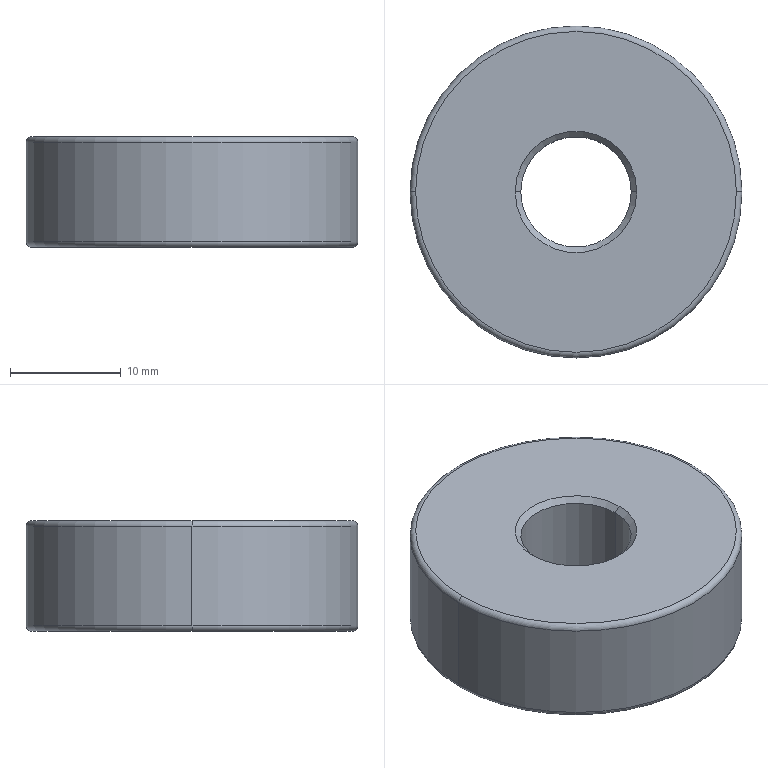Part | SolidWorks | features MirrorStock 1 | 1 solid | 14 faces | box 30 x 30 x 10 mm | volume 6265 mm3 | cone 4 | torus 4 | cylinder 4 | plane 2 | commonest cylinder face diameters 10 x2 30 x2
STEP:
#1=CARTESIAN_POINT('',(5.,0.,-9.5));
#2=VERTEX_POINT('',#1);
#3=CARTESIAN_POINT('',(-5.,0.,-9.5));
#4=VERTEX_POINT('',#3);
#5=CARTESIAN_POINT('',(0.,0.,-9.5));
#6=DIRECTION('',(0.,0.,1.));
#7=DIRECTION('',(1.,0.,0.));
#8=AXIS2_PLACEMENT_3D('',#5,#6,#7);
#9=CIRCLE('',#8,5.);
#10=EDGE_CURVE('',#2,#4,#9,.T.);
#11=ORIENTED_EDGE('',*,*,#10,.T.);
#12=CARTESIAN_POINT('',(-5.5,0.,-10.));
#13=VERTEX_POINT('',#12);
#14=CARTESIAN_POINT('',(-5.,0.,-9.5));
#15=DIRECTION('',(-0.7071,0.,-0.7071));
#16=VECTOR('',#15,1000.);
#17=LINE('',#14,#16);
#18=EDGE_CURVE('',#4,#13,#17,.T.);
#19=ORIENTED_EDGE('',*,*,#18,.T.);
#20=CARTESIAN_POINT('',(5.5,0.,-10.));
#21=VERTEX_POINT('',#20);
#22=CARTESIAN_POINT('',(0.,0.,-10.));
#23=DIRECTION('',(0.,0.,-1.));
#24=DIRECTION('',(1.,0.,0.));
#25=AXIS2_PLACEMENT_3D('',#22,#23,#24);
#26=CIRCLE('',#25,5.5);
#27=EDGE_CURVE('',#13,#21,#26,.T.);
#28=ORIENTED_EDGE('',*,*,#27,.T.);
#29=CARTESIAN_POINT('',(5.,0.,-9.5));
#30=DIRECTION('',(0.7071,0.,-0.7071));
#31=VECTOR('',#30,1000.);
#32=LINE('',#29,#31);
#33=EDGE_CURVE('',#2,#21,#32,.T.);
#34=ORIENTED_EDGE('',*,*,#33,.F.);
#35=EDGE_LOOP('',(#11,#19,#28,#34));
#36=FACE_OUTER_BOUND('',#35,.T.);
#37=CARTESIAN_POINT('',(0.,0.,-9.5));
#38=DIRECTION('',(0.,0.,-1.));
#39=DIRECTION('',(1.,0.,0.));
#40=AXIS2_PLACEMENT_3D('',#37,#38,#39);
#41=CONICAL_SURFACE('',#40,5.,0.7854);
#42=ADVANCED_FACE('',(#36),#41,.F.);
#43=CARTESIAN_POINT('',(-5.,0.,-0.5));
#44=VERTEX_POINT('',#43);
#45=CARTESIAN_POINT('',(5.,0.,-0.5));
#46=VERTEX_POINT('',#45);
#47=CARTESIAN_POINT('',(0.,0.,-0.5));
#48=DIRECTION('',(0.,0.,-1.));
#49=DIRECTION('',(1.,0.,0.));
#50=AXIS2_PLACEMENT_3D('',#47,#48,#49);
#51=CIRCLE('',#50,5.);
#52=EDGE_CURVE('',#44,#46,#51,.T.);
#53=ORIENTED_EDGE('',*,*,#52,.T.);
#54=CARTESIAN_POINT('',(5.5,0.,0.));
#55=VERTEX_POINT('',#54);
#56=CARTESIAN_POINT('',(5.5,0.,0.));
#57=DIRECTION('',(0.7071,0.,0.7071));
#58=VECTOR('',#57,1000.);
#59=LINE('',#56,#58);
#60=EDGE_CURVE('',#46,#55,#59,.T.);
#61=ORIENTED_EDGE('',*,*,#60,.T.);
#62=CARTESIAN_POINT('',(-5.5,0.,0.));
#63=VERTEX_POINT('',#62);
#64=CARTESIAN_POINT('',(0.,0.,0.));
#65=DIRECTION('',(0.,0.,1.));
#66=DIRECTION('',(1.,0.,0.));
#67=AXIS2_PLACEMENT_3D('',#64,#65,#66);
#68=CIRCLE('',#67,5.5);
#69=EDGE_CURVE('',#55,#63,#68,.T.);
#70=ORIENTED_EDGE('',*,*,#69,.T.);
#71=CARTESIAN_POINT('',(-5.5,0.,0.));
#72=DIRECTION('',(-0.7071,0.,0.7071));
#73=VECTOR('',#72,1000.);
#74=LINE('',#71,#73);
#75=EDGE_CURVE('',#44,#63,#74,.T.);
#76=ORIENTED_EDGE('',*,*,#75,.F.);
#77=EDGE_LOOP('',(#53,#61,#70,#76));
#78=FACE_OUTER_BOUND('',#77,.T.);
#79=CARTESIAN_POINT('',(0.,0.,0.));
#80=DIRECTION('',(0.,0.,1.));
#81=DIRECTION('',(-1.,0.,0.));
#82=AXIS2_PLACEMENT_3D('',#79,#80,#81);
#83=CONICAL_SURFACE('',#82,5.5,0.7854);
#84=ADVANCED_FACE('',(#78),#83,.F.);
#85=CARTESIAN_POINT('',(15.,0.,-9.5));
#86=VERTEX_POINT('',#85);
#87=CARTESIAN_POINT('',(-15.,0.,-9.5));
#88=VERTEX_POINT('',#87);
#89=CARTESIAN_POINT('',(0.,0.,-9.5));
#90=DIRECTION('',(0.,0.,-1.));
#91=DIRECTION('',(1.,0.,0.));
#92=AXIS2_PLACEMENT_3D('',#89,#90,#91);
#93=CIRCLE('',#92,15.);
#94=EDGE_CURVE('',#86,#88,#93,.T.);
#95=ORIENTED_EDGE('',*,*,#94,.T.);
#96=CARTESIAN_POINT('',(-14.5,0.,-10.));
#97=VERTEX_POINT('',#96);
#98=CARTESIAN_POINT('',(-14.5,0.,-9.5));
#99=DIRECTION('',(0.,-1.,0.));
#100=DIRECTION('',(1.,0.,0.));
#101=AXIS2_PLACEMENT_3D('',#98,#99,#100);
#102=CIRCLE('',#101,0.5);
#103=EDGE_CURVE('',#88,#97,#102,.T.);
#104=ORIENTED_EDGE('',*,*,#103,.T.);
#105=CARTESIAN_POINT('',(14.5,0.,-10.));
#106=VERTEX_POINT('',#105);
#107=CARTESIAN_POINT('',(0.,0.,-10.));
#108=DIRECTION('',(0.,0.,1.));
#109=DIRECTION('',(1.,0.,0.));
#110=AXIS2_PLACEMENT_3D('',#107,#108,#109);
#111=CIRCLE('',#110,14.5);
#112=EDGE_CURVE('',#97,#106,#111,.T.);
#113=ORIENTED_EDGE('',*,*,#112,.T.);
#114=CARTESIAN_POINT('',(14.5,0.,-9.5));
#115=DIRECTION('',(0.,1.,0.));
#116=DIRECTION('',(-1.,0.,0.));
#117=AXIS2_PLACEMENT_3D('',#114,#115,#116);
#118=CIRCLE('',#117,0.5);
#119=EDGE_CURVE('',#86,#106,#118,.T.);
#120=ORIENTED_EDGE('',*,*,#119,.F.);
#121=EDGE_LOOP('',(#95,#104,#113,#120));
#122=FACE_OUTER_BOUND('',#121,.T.);
#123=CARTESIAN_POINT('',(0.,0.,-9.5));
#124=DIRECTION('',(0.,0.,-1.));
#125=DIRECTION('',(1.,0.,0.));
#126=AXIS2_PLACEMENT_3D('',#123,#124,#125);
#127=TOROIDAL_SURFACE('',#126,14.5,0.5);
#128=ADVANCED_FACE('',(#122),#127,.T.);
#129=CARTESIAN_POINT('',(14.5,0.,0.));
#130=VERTEX_POINT('',#129);
#131=CARTESIAN_POINT('',(-14.5,0.,0.));
#132=VERTEX_POINT('',#131);
#133=CARTESIAN_POINT('',(0.,0.,0.));
#134=DIRECTION('',(0.,0.,-1.));
#135=DIRECTION('',(1.,0.,0.));
#136=AXIS2_PLACEMENT_3D('',#133,#134,#135);
#137=CIRCLE('',#136,14.5);
#138=EDGE_CURVE('',#130,#132,#137,.T.);
#139=ORIENTED_EDGE('',*,*,#138,.T.);
#140=CARTESIAN_POINT('',(-15.,0.,-0.5));
#141=VERTEX_POINT('',#140);
#142=CARTESIAN_POINT('',(-14.5,0.,-0.5));
#143=DIRECTION('',(0.,-1.,0.));
#144=DIRECTION('',(1.,0.,0.));
#145=AXIS2_PLACEMENT_3D('',#142,#143,#144);
#146=CIRCLE('',#145,0.5);
#147=EDGE_CURVE('',#132,#141,#146,.T.);
#148=ORIENTED_EDGE('',*,*,#147,.T.);
#149=CARTESIAN_POINT('',(15.,0.,-0.5));
#150=VERTEX_POINT('',#149);
#151=CARTESIAN_POINT('',(0.,0.,-0.5));
#152=DIRECTION('',(0.,0.,1.));
#153=DIRECTION('',(1.,0.,0.));
#154=AXIS2_PLACEMENT_3D('',#151,#152,#153);
#155=CIRCLE('',#154,15.);
#156=EDGE_CURVE('',#141,#150,#155,.T.);
#157=ORIENTED_EDGE('',*,*,#156,.T.);
#158=CARTESIAN_POINT('',(14.5,0.,-0.5));
#159=DIRECTION('',(0.,1.,0.));
#160=DIRECTION('',(-1.,0.,0.));
#161=AXIS2_PLACEMENT_3D('',#158,#159,#160);
#162=CIRCLE('',#161,0.5);
#163=EDGE_CURVE('',#130,#150,#162,.T.);
#164=ORIENTED_EDGE('',*,*,#163,.F.);
#165=EDGE_LOOP('',(#139,#148,#157,#164));
#166=FACE_OUTER_BOUND('',#165,.T.);
#167=CARTESIAN_POINT('',(0.,0.,-0.5));
#168=DIRECTION('',(0.,0.,-1.));
#169=DIRECTION('',(1.,0.,0.));
#170=AXIS2_PLACEMENT_3D('',#167,#168,#169);
#171=TOROIDAL_SURFACE('',#170,14.5,0.5);
#172=ADVANCED_FACE('',(#166),#171,.T.);
#173=ORIENTED_EDGE('',*,*,#10,.F.);
#174=CARTESIAN_POINT('',(5.,0.,-10.));
#175=DIRECTION('',(0.,0.,1.));
#176=VECTOR('',#175,1000.);
#177=LINE('',#174,#176);
#178=EDGE_CURVE('',#2,#46,#177,.T.);
#179=ORIENTED_EDGE('',*,*,#178,.T.);
#180=ORIENTED_EDGE('',*,*,#52,.F.);
#181=CARTESIAN_POINT('',(-5.,0.,-10.));
#182=DIRECTION('',(0.,0.,1.));
#183=VECTOR('',#182,1000.);
#184=LINE('',#181,#183);
#185=EDGE_CURVE('',#4,#44,#184,.T.);
#186=ORIENTED_EDGE('',*,*,#185,.F.);
#187=EDGE_LOOP('',(#173,#179,#180,#186));
#188=FACE_OUTER_BOUND('',#187,.T.);
#189=CARTESIAN_POINT('',(0.,0.,-10.));
#190=DIRECTION('',(0.,0.,1.));
#191=DIRECTION('',(-1.,0.,0.));
#192=AXIS2_PLACEMENT_3D('',#189,#190,#191);
#193=CYLINDRICAL_SURFACE('',#192,5.);
#194=ADVANCED_FACE('',(#188),#193,.F.);
#195=ORIENTED_EDGE('',*,*,#94,.F.);
#196=CARTESIAN_POINT('',(15.,0.,-10.));
#197=DIRECTION('',(0.,0.,1.));
#198=VECTOR('',#197,1000.);
#199=LINE('',#196,#198);
#200=EDGE_CURVE('',#86,#150,#199,.T.);
#201=ORIENTED_EDGE('',*,*,#200,.T.);
#202=ORIENTED_EDGE('',*,*,#156,.F.);
#203=CARTESIAN_POINT('',(-15.,0.,-10.));
#204=DIRECTION('',(0.,0.,1.));
#205=VECTOR('',#204,1000.);
#206=LINE('',#203,#205);
#207=EDGE_CURVE('',#88,#141,#206,.T.);
#208=ORIENTED_EDGE('',*,*,#207,.F.);
#209=EDGE_LOOP('',(#195,#201,#202,#208));
#210=FACE_OUTER_BOUND('',#209,.T.);
#211=CARTESIAN_POINT('',(0.,0.,-10.));
#212=DIRECTION('',(0.,0.,1.));
#213=DIRECTION('',(-1.,0.,0.));
#214=AXIS2_PLACEMENT_3D('',#211,#212,#213);
#215=CYLINDRICAL_SURFACE('',#214,15.);
#216=ADVANCED_FACE('',(#210),#215,.T.);
#217=CARTESIAN_POINT('',(0.,0.,-10.));
#218=DIRECTION('',(0.,0.,-1.));
#219=DIRECTION('',(1.,0.,0.));
#220=AXIS2_PLACEMENT_3D('',#217,#218,#219);
#221=CIRCLE('',#220,5.5);
#222=EDGE_CURVE('',#21,#13,#221,.T.);
#223=ORIENTED_EDGE('',*,*,#222,.F.);
#224=ORIENTED_EDGE('',*,*,#27,.F.);
#225=EDGE_LOOP('',(#223,#224));
#226=FACE_BOUND('',#225,.T.);
#227=CARTESIAN_POINT('',(0.,0.,-10.));
#228=DIRECTION('',(0.,0.,1.));
#229=DIRECTION('',(1.,0.,0.));
#230=AXIS2_PLACEMENT_3D('',#227,#228,#229);
#231=CIRCLE('',#230,14.5);
#232=EDGE_CURVE('',#106,#97,#231,.T.);
#233=ORIENTED_EDGE('',*,*,#232,.F.);
#234=ORIENTED_EDGE('',*,*,#112,.F.);
#235=EDGE_LOOP('',(#233,#234));
#236=FACE_OUTER_BOUND('',#235,.T.);
#237=CARTESIAN_POINT('',(0.,0.,-10.));
#238=DIRECTION('',(0.,0.,-1.));
#239=DIRECTION('',(1.,0.,0.));
#240=AXIS2_PLACEMENT_3D('',#237,#238,#239);
#241=PLANE('',#240);
#242=ADVANCED_FACE('',(#226,#236),#241,.T.);
#243=CARTESIAN_POINT('',(0.,0.,0.));
#244=DIRECTION('',(0.,0.,1.));
#245=DIRECTION('',(1.,0.,0.));
#246=AXIS2_PLACEMENT_3D('',#243,#244,#245);
#247=CIRCLE('',#246,5.5);
#248=EDGE_CURVE('',#63,#55,#247,.T.);
#249=ORIENTED_EDGE('',*,*,#248,.F.);
#250=ORIENTED_EDGE('',*,*,#69,.F.);
#251=EDGE_LOOP('',(#249,#250));
#252=FACE_BOUND('',#251,.T.);
#253=ORIENTED_EDGE('',*,*,#138,.F.);
#254=CARTESIAN_POINT('',(0.,0.,0.));
#255=DIRECTION('',(0.,0.,-1.));
#256=DIRECTION('',(1.,0.,0.));
#257=AXIS2_PLACEMENT_3D('',#254,#255,#256);
#258=CIRCLE('',#257,14.5);
#259=EDGE_CURVE('',#132,#130,#258,.T.);
#260=ORIENTED_EDGE('',*,*,#259,.F.);
#261=EDGE_LOOP('',(#253,#260));
#262=FACE_OUTER_BOUND('',#261,.T.);
#263=CARTESIAN_POINT('',(0.,0.,0.));
#264=DIRECTION('',(0.,0.,-1.));
#265=DIRECTION('',(1.,0.,0.));
#266=AXIS2_PLACEMENT_3D('',#263,#264,#265);
#267=PLANE('',#266);
#268=ADVANCED_FACE('',(#252,#262),#267,.F.);
#269=ORIENTED_EDGE('',*,*,#200,.F.);
#270=CARTESIAN_POINT('',(0.,0.,-9.5));
#271=DIRECTION('',(0.,0.,-1.));
#272=DIRECTION('',(1.,0.,0.));
#273=AXIS2_PLACEMENT_3D('',#270,#271,#272);
#274=CIRCLE('',#273,15.);
#275=EDGE_CURVE('',#88,#86,#274,.T.);
#276=ORIENTED_EDGE('',*,*,#275,.F.);
#277=ORIENTED_EDGE('',*,*,#207,.T.);
#278=CARTESIAN_POINT('',(0.,0.,-0.5));
#279=DIRECTION('',(0.,0.,1.));
#280=DIRECTION('',(1.,0.,0.));
#281=AXIS2_PLACEMENT_3D('',#278,#279,#280);
#282=CIRCLE('',#281,15.);
#283=EDGE_CURVE('',#150,#141,#282,.T.);
#284=ORIENTED_EDGE('',*,*,#283,.F.);
#285=EDGE_LOOP('',(#269,#276,#277,#284));
#286=FACE_OUTER_BOUND('',#285,.T.);
#287=CARTESIAN_POINT('',(0.,0.,-10.));
#288=DIRECTION('',(0.,0.,1.));
#289=DIRECTION('',(-1.,0.,0.));
#290=AXIS2_PLACEMENT_3D('',#287,#288,#289);
#291=CYLINDRICAL_SURFACE('',#290,15.);
#292=ADVANCED_FACE('',(#286),#291,.T.);
#293=ORIENTED_EDGE('',*,*,#178,.F.);
#294=CARTESIAN_POINT('',(0.,0.,-9.5));
#295=DIRECTION('',(0.,0.,1.));
#296=DIRECTION('',(1.,0.,0.));
#297=AXIS2_PLACEMENT_3D('',#294,#295,#296);
#298=CIRCLE('',#297,5.);
#299=EDGE_CURVE('',#4,#2,#298,.T.);
#300=ORIENTED_EDGE('',*,*,#299,.F.);
#301=ORIENTED_EDGE('',*,*,#185,.T.);
#302=CARTESIAN_POINT('',(0.,0.,-0.5));
#303=DIRECTION('',(0.,0.,-1.));
#304=DIRECTION('',(1.,0.,0.));
#305=AXIS2_PLACEMENT_3D('',#302,#303,#304);
#306=CIRCLE('',#305,5.);
#307=EDGE_CURVE('',#46,#44,#306,.T.);
#308=ORIENTED_EDGE('',*,*,#307,.F.);
#309=EDGE_LOOP('',(#293,#300,#301,#308));
#310=FACE_OUTER_BOUND('',#309,.T.);
#311=CARTESIAN_POINT('',(0.,0.,-10.));
#312=DIRECTION('',(0.,0.,1.));
#313=DIRECTION('',(-1.,0.,0.));
#314=AXIS2_PLACEMENT_3D('',#311,#312,#313);
#315=CYLINDRICAL_SURFACE('',#314,5.);
#316=ADVANCED_FACE('',(#310),#315,.F.);
#317=ORIENTED_EDGE('',*,*,#147,.F.);
#318=ORIENTED_EDGE('',*,*,#259,.T.);
#319=ORIENTED_EDGE('',*,*,#163,.T.);
#320=ORIENTED_EDGE('',*,*,#283,.T.);
#321=EDGE_LOOP('',(#317,#318,#319,#320));
#322=FACE_OUTER_BOUND('',#321,.T.);
#323=CARTESIAN_POINT('',(0.,0.,-0.5));
#324=DIRECTION('',(0.,0.,-1.));
#325=DIRECTION('',(1.,0.,0.));
#326=AXIS2_PLACEMENT_3D('',#323,#324,#325);
#327=TOROIDAL_SURFACE('',#326,14.5,0.5);
#328=ADVANCED_FACE('',(#322),#327,.T.);
#329=ORIENTED_EDGE('',*,*,#103,.F.);
#330=ORIENTED_EDGE('',*,*,#275,.T.);
#331=ORIENTED_EDGE('',*,*,#119,.T.);
#332=ORIENTED_EDGE('',*,*,#232,.T.);
#333=EDGE_LOOP('',(#329,#330,#331,#332));
#334=FACE_OUTER_BOUND('',#333,.T.);
#335=CARTESIAN_POINT('',(0.,0.,-9.5));
#336=DIRECTION('',(0.,0.,-1.));
#337=DIRECTION('',(1.,0.,0.));
#338=AXIS2_PLACEMENT_3D('',#335,#336,#337);
#339=TOROIDAL_SURFACE('',#338,14.5,0.5);
#340=ADVANCED_FACE('',(#334),#339,.T.);
#341=ORIENTED_EDGE('',*,*,#60,.F.);
#342=ORIENTED_EDGE('',*,*,#307,.T.);
#343=ORIENTED_EDGE('',*,*,#75,.T.);
#344=ORIENTED_EDGE('',*,*,#248,.T.);
#345=EDGE_LOOP('',(#341,#342,#343,#344));
#346=FACE_OUTER_BOUND('',#345,.T.);
#347=CARTESIAN_POINT('',(0.,0.,0.));
#348=DIRECTION('',(0.,0.,1.));
#349=DIRECTION('',(-1.,0.,0.));
#350=AXIS2_PLACEMENT_3D('',#347,#348,#349);
#351=CONICAL_SURFACE('',#350,5.5,0.7854);
#352=ADVANCED_FACE('',(#346),#351,.F.);
#353=ORIENTED_EDGE('',*,*,#18,.F.);
#354=ORIENTED_EDGE('',*,*,#299,.T.);
#355=ORIENTED_EDGE('',*,*,#33,.T.);
#356=ORIENTED_EDGE('',*,*,#222,.T.);
#357=EDGE_LOOP('',(#353,#354,#355,#356));
#358=FACE_OUTER_BOUND('',#357,.T.);
#359=CARTESIAN_POINT('',(0.,0.,-9.5));
#360=DIRECTION('',(0.,0.,-1.));
#361=DIRECTION('',(1.,0.,0.));
#362=AXIS2_PLACEMENT_3D('',#359,#360,#361);
#363=CONICAL_SURFACE('',#362,5.,0.7854);
#364=ADVANCED_FACE('',(#358),#363,.F.);
#365=CLOSED_SHELL('',(#42,#84,#128,#172,#194,#216,#242,#268,#292,#316,#328,#340,#352,#364));
#366=MANIFOLD_SOLID_BREP('',#365);
#367=CARTESIAN_POINT('',(0.,0.,0.));
#368=DIRECTION('',(0.,0.,1.));
#369=DIRECTION('',(1.,0.,0.));
#370=AXIS2_PLACEMENT_3D('',#367,#368,#369);
#371=(LENGTH_UNIT()NAMED_UNIT(*)SI_UNIT(.MILLI.,.METRE.));
#372=UNCERTAINTY_MEASURE_WITH_UNIT(LENGTH_MEASURE(0.00001),#371,'','');
#373=(NAMED_UNIT(*)PLANE_ANGLE_UNIT()SI_UNIT($,.RADIAN.));
#374=(NAMED_UNIT(*)SI_UNIT($,.STERADIAN.)SOLID_ANGLE_UNIT());
#375=(GEOMETRIC_REPRESENTATION_CONTEXT(3)GLOBAL_UNCERTAINTY_ASSIGNED_CONTEXT((#372))GLOBAL_UNIT_ASSIGNED_CONTEXT((#371,#373,#374))REPRESENTATION_CONTEXT('',''));
#376=ADVANCED_BREP_SHAPE_REPRESENTATION('',(#366,#370),#375);